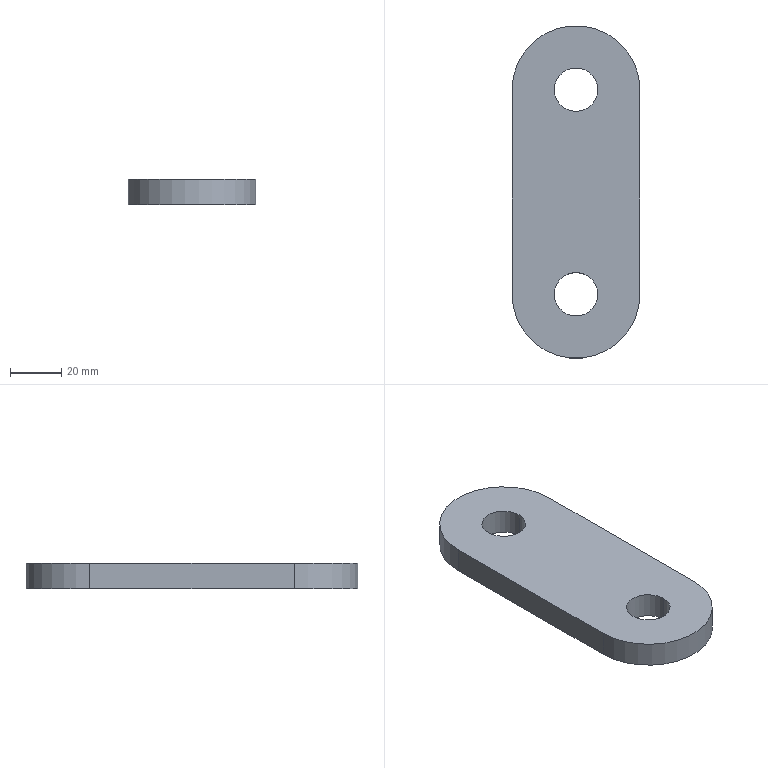Part | SolidWorks | features Extrusion 1 | 1 solid | 10 faces | box 50 x 130 x 10 mm | volume 55095 mm3 | cylinder 6 | plane 4 | commonest cylinder face diameters 17 x4 50 x2
STEP:
#1=CARTESIAN_POINT('',(-8.5,80.,10.));
#2=VERTEX_POINT('',#1);
#3=CARTESIAN_POINT('',(8.5,80.,10.));
#4=VERTEX_POINT('',#3);
#5=CARTESIAN_POINT('',(0.,80.,10.));
#6=DIRECTION('',(0.,0.,1.));
#7=DIRECTION('',(1.,0.,0.));
#8=AXIS2_PLACEMENT_3D('',#5,#6,#7);
#9=CIRCLE('',#8,8.5);
#10=EDGE_CURVE('',#2,#4,#9,.T.);
#11=ORIENTED_EDGE('',*,*,#10,.T.);
#12=CARTESIAN_POINT('',(8.5,80.,0.));
#13=VERTEX_POINT('',#12);
#14=CARTESIAN_POINT('',(8.5,80.,10.));
#15=DIRECTION('',(0.,0.,-1.));
#16=VECTOR('',#15,1000.);
#17=LINE('',#14,#16);
#18=EDGE_CURVE('',#4,#13,#17,.T.);
#19=ORIENTED_EDGE('',*,*,#18,.T.);
#20=CARTESIAN_POINT('',(-8.5,80.,0.));
#21=VERTEX_POINT('',#20);
#22=CARTESIAN_POINT('',(0.,80.,0.));
#23=DIRECTION('',(0.,0.,1.));
#24=DIRECTION('',(1.,0.,0.));
#25=AXIS2_PLACEMENT_3D('',#22,#23,#24);
#26=CIRCLE('',#25,8.5);
#27=EDGE_CURVE('',#21,#13,#26,.T.);
#28=ORIENTED_EDGE('',*,*,#27,.F.);
#29=CARTESIAN_POINT('',(-8.5,80.,10.));
#30=DIRECTION('',(0.,0.,-1.));
#31=VECTOR('',#30,1000.);
#32=LINE('',#29,#31);
#33=EDGE_CURVE('',#2,#21,#32,.T.);
#34=ORIENTED_EDGE('',*,*,#33,.F.);
#35=EDGE_LOOP('',(#11,#19,#28,#34));
#36=FACE_OUTER_BOUND('',#35,.T.);
#37=CARTESIAN_POINT('',(0.,80.,10.));
#38=DIRECTION('',(0.,0.,-1.));
#39=DIRECTION('',(-1.,0.,0.));
#40=AXIS2_PLACEMENT_3D('',#37,#38,#39);
#41=CYLINDRICAL_SURFACE('',#40,8.5);
#42=ADVANCED_FACE('',(#36),#41,.F.);
#43=CARTESIAN_POINT('',(-8.5,0.,10.));
#44=VERTEX_POINT('',#43);
#45=CARTESIAN_POINT('',(8.5,0.,10.));
#46=VERTEX_POINT('',#45);
#47=CARTESIAN_POINT('',(0.,0.,10.));
#48=DIRECTION('',(0.,0.,1.));
#49=DIRECTION('',(1.,0.,0.));
#50=AXIS2_PLACEMENT_3D('',#47,#48,#49);
#51=CIRCLE('',#50,8.5);
#52=EDGE_CURVE('',#44,#46,#51,.T.);
#53=ORIENTED_EDGE('',*,*,#52,.T.);
#54=CARTESIAN_POINT('',(8.5,0.,0.));
#55=VERTEX_POINT('',#54);
#56=CARTESIAN_POINT('',(8.5,0.,10.));
#57=DIRECTION('',(0.,0.,-1.));
#58=VECTOR('',#57,1000.);
#59=LINE('',#56,#58);
#60=EDGE_CURVE('',#46,#55,#59,.T.);
#61=ORIENTED_EDGE('',*,*,#60,.T.);
#62=CARTESIAN_POINT('',(-8.5,0.,0.));
#63=VERTEX_POINT('',#62);
#64=CARTESIAN_POINT('',(0.,0.,0.));
#65=DIRECTION('',(0.,0.,1.));
#66=DIRECTION('',(1.,0.,0.));
#67=AXIS2_PLACEMENT_3D('',#64,#65,#66);
#68=CIRCLE('',#67,8.5);
#69=EDGE_CURVE('',#63,#55,#68,.T.);
#70=ORIENTED_EDGE('',*,*,#69,.F.);
#71=CARTESIAN_POINT('',(-8.5,0.,10.));
#72=DIRECTION('',(0.,0.,-1.));
#73=VECTOR('',#72,1000.);
#74=LINE('',#71,#73);
#75=EDGE_CURVE('',#44,#63,#74,.T.);
#76=ORIENTED_EDGE('',*,*,#75,.F.);
#77=EDGE_LOOP('',(#53,#61,#70,#76));
#78=FACE_OUTER_BOUND('',#77,.T.);
#79=CARTESIAN_POINT('',(0.,0.,10.));
#80=DIRECTION('',(0.,0.,-1.));
#81=DIRECTION('',(-1.,0.,0.));
#82=AXIS2_PLACEMENT_3D('',#79,#80,#81);
#83=CYLINDRICAL_SURFACE('',#82,8.5);
#84=ADVANCED_FACE('',(#78),#83,.F.);
#85=ORIENTED_EDGE('',*,*,#52,.F.);
#86=CARTESIAN_POINT('',(0.,0.,10.));
#87=DIRECTION('',(0.,0.,1.));
#88=DIRECTION('',(1.,0.,0.));
#89=AXIS2_PLACEMENT_3D('',#86,#87,#88);
#90=CIRCLE('',#89,8.5);
#91=EDGE_CURVE('',#46,#44,#90,.T.);
#92=ORIENTED_EDGE('',*,*,#91,.F.);
#93=EDGE_LOOP('',(#85,#92));
#94=FACE_BOUND('',#93,.T.);
#95=CARTESIAN_POINT('',(-25.,0.,10.));
#96=VERTEX_POINT('',#95);
#97=CARTESIAN_POINT('',(25.,0.,10.));
#98=VERTEX_POINT('',#97);
#99=CARTESIAN_POINT('',(0.,0.,10.));
#100=DIRECTION('',(0.,0.,1.));
#101=DIRECTION('',(1.,0.,0.));
#102=AXIS2_PLACEMENT_3D('',#99,#100,#101);
#103=CIRCLE('',#102,25.);
#104=EDGE_CURVE('',#96,#98,#103,.T.);
#105=ORIENTED_EDGE('',*,*,#104,.T.);
#106=CARTESIAN_POINT('',(25.,80.,10.));
#107=VERTEX_POINT('',#106);
#108=CARTESIAN_POINT('',(25.,0.,10.));
#109=DIRECTION('',(0.,1.,0.));
#110=VECTOR('',#109,1000.);
#111=LINE('',#108,#110);
#112=EDGE_CURVE('',#98,#107,#111,.T.);
#113=ORIENTED_EDGE('',*,*,#112,.T.);
#114=CARTESIAN_POINT('',(-25.,80.,10.));
#115=VERTEX_POINT('',#114);
#116=CARTESIAN_POINT('',(0.,80.,10.));
#117=DIRECTION('',(0.,0.,1.));
#118=DIRECTION('',(1.,0.,0.));
#119=AXIS2_PLACEMENT_3D('',#116,#117,#118);
#120=CIRCLE('',#119,25.);
#121=EDGE_CURVE('',#107,#115,#120,.T.);
#122=ORIENTED_EDGE('',*,*,#121,.T.);
#123=CARTESIAN_POINT('',(-25.,0.,10.));
#124=DIRECTION('',(0.,-1.,0.));
#125=VECTOR('',#124,1000.);
#126=LINE('',#123,#125);
#127=EDGE_CURVE('',#115,#96,#126,.T.);
#128=ORIENTED_EDGE('',*,*,#127,.T.);
#129=EDGE_LOOP('',(#105,#113,#122,#128));
#130=FACE_OUTER_BOUND('',#129,.T.);
#131=ORIENTED_EDGE('',*,*,#10,.F.);
#132=CARTESIAN_POINT('',(0.,80.,10.));
#133=DIRECTION('',(0.,0.,1.));
#134=DIRECTION('',(1.,0.,0.));
#135=AXIS2_PLACEMENT_3D('',#132,#133,#134);
#136=CIRCLE('',#135,8.5);
#137=EDGE_CURVE('',#4,#2,#136,.T.);
#138=ORIENTED_EDGE('',*,*,#137,.F.);
#139=EDGE_LOOP('',(#131,#138));
#140=FACE_BOUND('',#139,.T.);
#141=CARTESIAN_POINT('',(0.,0.,10.));
#142=DIRECTION('',(0.,0.,1.));
#143=DIRECTION('',(1.,0.,0.));
#144=AXIS2_PLACEMENT_3D('',#141,#142,#143);
#145=PLANE('',#144);
#146=ADVANCED_FACE('',(#94,#130,#140),#145,.T.);
#147=CARTESIAN_POINT('',(-25.,0.,0.));
#148=VERTEX_POINT('',#147);
#149=CARTESIAN_POINT('',(25.,0.,0.));
#150=VERTEX_POINT('',#149);
#151=CARTESIAN_POINT('',(0.,0.,0.));
#152=DIRECTION('',(0.,0.,1.));
#153=DIRECTION('',(1.,0.,0.));
#154=AXIS2_PLACEMENT_3D('',#151,#152,#153);
#155=CIRCLE('',#154,25.);
#156=EDGE_CURVE('',#148,#150,#155,.T.);
#157=ORIENTED_EDGE('',*,*,#156,.F.);
#158=CARTESIAN_POINT('',(-25.,80.,0.));
#159=VERTEX_POINT('',#158);
#160=CARTESIAN_POINT('',(-25.,0.,0.));
#161=DIRECTION('',(0.,-1.,0.));
#162=VECTOR('',#161,1000.);
#163=LINE('',#160,#162);
#164=EDGE_CURVE('',#159,#148,#163,.T.);
#165=ORIENTED_EDGE('',*,*,#164,.F.);
#166=CARTESIAN_POINT('',(25.,80.,0.));
#167=VERTEX_POINT('',#166);
#168=CARTESIAN_POINT('',(0.,80.,0.));
#169=DIRECTION('',(0.,0.,1.));
#170=DIRECTION('',(1.,0.,0.));
#171=AXIS2_PLACEMENT_3D('',#168,#169,#170);
#172=CIRCLE('',#171,25.);
#173=EDGE_CURVE('',#167,#159,#172,.T.);
#174=ORIENTED_EDGE('',*,*,#173,.F.);
#175=CARTESIAN_POINT('',(25.,0.,0.));
#176=DIRECTION('',(0.,1.,0.));
#177=VECTOR('',#176,1000.);
#178=LINE('',#175,#177);
#179=EDGE_CURVE('',#150,#167,#178,.T.);
#180=ORIENTED_EDGE('',*,*,#179,.F.);
#181=EDGE_LOOP('',(#157,#165,#174,#180));
#182=FACE_OUTER_BOUND('',#181,.T.);
#183=ORIENTED_EDGE('',*,*,#69,.T.);
#184=CARTESIAN_POINT('',(0.,0.,0.));
#185=DIRECTION('',(0.,0.,1.));
#186=DIRECTION('',(1.,0.,0.));
#187=AXIS2_PLACEMENT_3D('',#184,#185,#186);
#188=CIRCLE('',#187,8.5);
#189=EDGE_CURVE('',#55,#63,#188,.T.);
#190=ORIENTED_EDGE('',*,*,#189,.T.);
#191=EDGE_LOOP('',(#183,#190));
#192=FACE_BOUND('',#191,.T.);
#193=ORIENTED_EDGE('',*,*,#27,.T.);
#194=CARTESIAN_POINT('',(0.,80.,0.));
#195=DIRECTION('',(0.,0.,1.));
#196=DIRECTION('',(1.,0.,0.));
#197=AXIS2_PLACEMENT_3D('',#194,#195,#196);
#198=CIRCLE('',#197,8.5);
#199=EDGE_CURVE('',#13,#21,#198,.T.);
#200=ORIENTED_EDGE('',*,*,#199,.T.);
#201=EDGE_LOOP('',(#193,#200));
#202=FACE_BOUND('',#201,.T.);
#203=CARTESIAN_POINT('',(0.,0.,0.));
#204=DIRECTION('',(0.,0.,1.));
#205=DIRECTION('',(1.,0.,0.));
#206=AXIS2_PLACEMENT_3D('',#203,#204,#205);
#207=PLANE('',#206);
#208=ADVANCED_FACE('',(#182,#192,#202),#207,.F.);
#209=ORIENTED_EDGE('',*,*,#156,.T.);
#210=CARTESIAN_POINT('',(25.,0.,10.));
#211=DIRECTION('',(0.,0.,-1.));
#212=VECTOR('',#211,1000.);
#213=LINE('',#210,#212);
#214=EDGE_CURVE('',#98,#150,#213,.T.);
#215=ORIENTED_EDGE('',*,*,#214,.F.);
#216=ORIENTED_EDGE('',*,*,#104,.F.);
#217=CARTESIAN_POINT('',(-25.,0.,10.));
#218=DIRECTION('',(0.,0.,-1.));
#219=VECTOR('',#218,1000.);
#220=LINE('',#217,#219);
#221=EDGE_CURVE('',#96,#148,#220,.T.);
#222=ORIENTED_EDGE('',*,*,#221,.T.);
#223=EDGE_LOOP('',(#209,#215,#216,#222));
#224=FACE_OUTER_BOUND('',#223,.T.);
#225=CARTESIAN_POINT('',(0.,0.,10.));
#226=DIRECTION('',(0.,0.,-1.));
#227=DIRECTION('',(-1.,0.,0.));
#228=AXIS2_PLACEMENT_3D('',#225,#226,#227);
#229=CYLINDRICAL_SURFACE('',#228,25.);
#230=ADVANCED_FACE('',(#224),#229,.T.);
#231=ORIENTED_EDGE('',*,*,#179,.T.);
#232=CARTESIAN_POINT('',(25.,80.,10.));
#233=DIRECTION('',(0.,0.,-1.));
#234=VECTOR('',#233,1000.);
#235=LINE('',#232,#234);
#236=EDGE_CURVE('',#107,#167,#235,.T.);
#237=ORIENTED_EDGE('',*,*,#236,.F.);
#238=ORIENTED_EDGE('',*,*,#112,.F.);
#239=ORIENTED_EDGE('',*,*,#214,.T.);
#240=EDGE_LOOP('',(#231,#237,#238,#239));
#241=FACE_OUTER_BOUND('',#240,.T.);
#242=CARTESIAN_POINT('',(25.,0.,10.));
#243=DIRECTION('',(-1.,0.,0.));
#244=DIRECTION('',(0.,0.,1.));
#245=AXIS2_PLACEMENT_3D('',#242,#243,#244);
#246=PLANE('',#245);
#247=ADVANCED_FACE('',(#241),#246,.F.);
#248=ORIENTED_EDGE('',*,*,#173,.T.);
#249=CARTESIAN_POINT('',(-25.,80.,10.));
#250=DIRECTION('',(0.,0.,-1.));
#251=VECTOR('',#250,1000.);
#252=LINE('',#249,#251);
#253=EDGE_CURVE('',#115,#159,#252,.T.);
#254=ORIENTED_EDGE('',*,*,#253,.F.);
#255=ORIENTED_EDGE('',*,*,#121,.F.);
#256=ORIENTED_EDGE('',*,*,#236,.T.);
#257=EDGE_LOOP('',(#248,#254,#255,#256));
#258=FACE_OUTER_BOUND('',#257,.T.);
#259=CARTESIAN_POINT('',(0.,80.,10.));
#260=DIRECTION('',(0.,0.,-1.));
#261=DIRECTION('',(-1.,0.,0.));
#262=AXIS2_PLACEMENT_3D('',#259,#260,#261);
#263=CYLINDRICAL_SURFACE('',#262,25.);
#264=ADVANCED_FACE('',(#258),#263,.T.);
#265=ORIENTED_EDGE('',*,*,#164,.T.);
#266=ORIENTED_EDGE('',*,*,#221,.F.);
#267=ORIENTED_EDGE('',*,*,#127,.F.);
#268=ORIENTED_EDGE('',*,*,#253,.T.);
#269=EDGE_LOOP('',(#265,#266,#267,#268));
#270=FACE_OUTER_BOUND('',#269,.T.);
#271=CARTESIAN_POINT('',(-25.,0.,10.));
#272=DIRECTION('',(1.,0.,0.));
#273=DIRECTION('',(0.,0.,-1.));
#274=AXIS2_PLACEMENT_3D('',#271,#272,#273);
#275=PLANE('',#274);
#276=ADVANCED_FACE('',(#270),#275,.F.);
#277=ORIENTED_EDGE('',*,*,#60,.F.);
#278=ORIENTED_EDGE('',*,*,#91,.T.);
#279=ORIENTED_EDGE('',*,*,#75,.T.);
#280=ORIENTED_EDGE('',*,*,#189,.F.);
#281=EDGE_LOOP('',(#277,#278,#279,#280));
#282=FACE_OUTER_BOUND('',#281,.T.);
#283=CARTESIAN_POINT('',(0.,0.,10.));
#284=DIRECTION('',(0.,0.,-1.));
#285=DIRECTION('',(-1.,0.,0.));
#286=AXIS2_PLACEMENT_3D('',#283,#284,#285);
#287=CYLINDRICAL_SURFACE('',#286,8.5);
#288=ADVANCED_FACE('',(#282),#287,.F.);
#289=ORIENTED_EDGE('',*,*,#18,.F.);
#290=ORIENTED_EDGE('',*,*,#137,.T.);
#291=ORIENTED_EDGE('',*,*,#33,.T.);
#292=ORIENTED_EDGE('',*,*,#199,.F.);
#293=EDGE_LOOP('',(#289,#290,#291,#292));
#294=FACE_OUTER_BOUND('',#293,.T.);
#295=CARTESIAN_POINT('',(0.,80.,10.));
#296=DIRECTION('',(0.,0.,-1.));
#297=DIRECTION('',(-1.,0.,0.));
#298=AXIS2_PLACEMENT_3D('',#295,#296,#297);
#299=CYLINDRICAL_SURFACE('',#298,8.5);
#300=ADVANCED_FACE('',(#294),#299,.F.);
#301=CLOSED_SHELL('',(#42,#84,#146,#208,#230,#247,#264,#276,#288,#300));
#302=MANIFOLD_SOLID_BREP('',#301);
#303=CARTESIAN_POINT('',(0.,0.,0.));
#304=DIRECTION('',(0.,0.,1.));
#305=DIRECTION('',(1.,0.,0.));
#306=AXIS2_PLACEMENT_3D('',#303,#304,#305);
#307=(LENGTH_UNIT()NAMED_UNIT(*)SI_UNIT(.MILLI.,.METRE.));
#308=UNCERTAINTY_MEASURE_WITH_UNIT(LENGTH_MEASURE(0.00001),#307,'','');
#309=(NAMED_UNIT(*)PLANE_ANGLE_UNIT()SI_UNIT($,.RADIAN.));
#310=(NAMED_UNIT(*)SI_UNIT($,.STERADIAN.)SOLID_ANGLE_UNIT());
#311=(GEOMETRIC_REPRESENTATION_CONTEXT(3)GLOBAL_UNCERTAINTY_ASSIGNED_CONTEXT((#308))GLOBAL_UNIT_ASSIGNED_CONTEXT((#307,#309,#310))REPRESENTATION_CONTEXT('',''));
#312=ADVANCED_BREP_SHAPE_REPRESENTATION('',(#302,#306),#311);